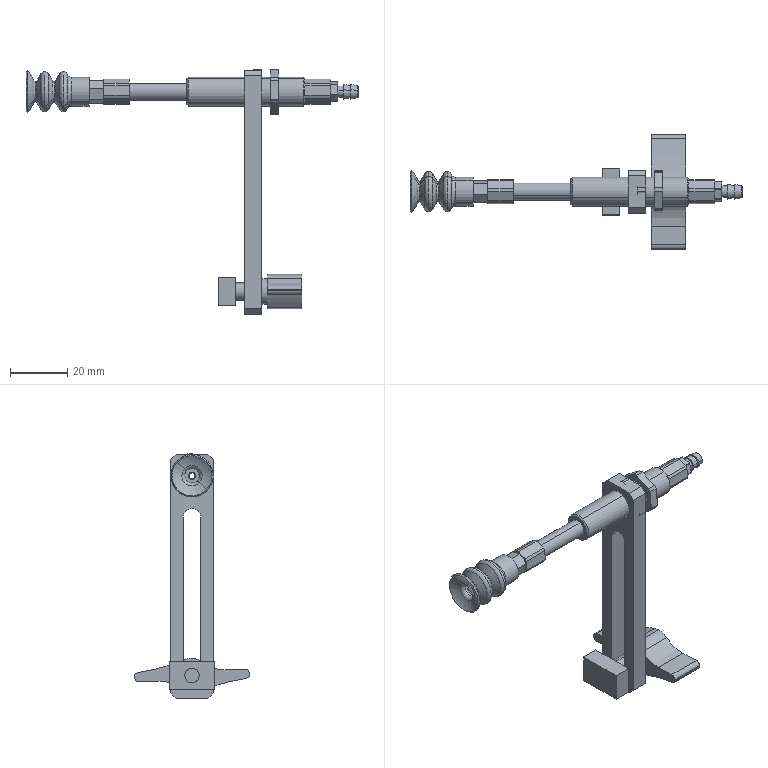Part | SolidWorks | 12 solids | 311 faces | box 115.5 x 39.995 x 85.247 mm | volume 15600 mm3 | plane 105 | cylinder 102 | cone 58 | torus 44 | sphere 2 | commonest cylinder face diameters 15.5 x16 8.7 x12 5 x10 0.6 x6 4.13 x6 9 x6